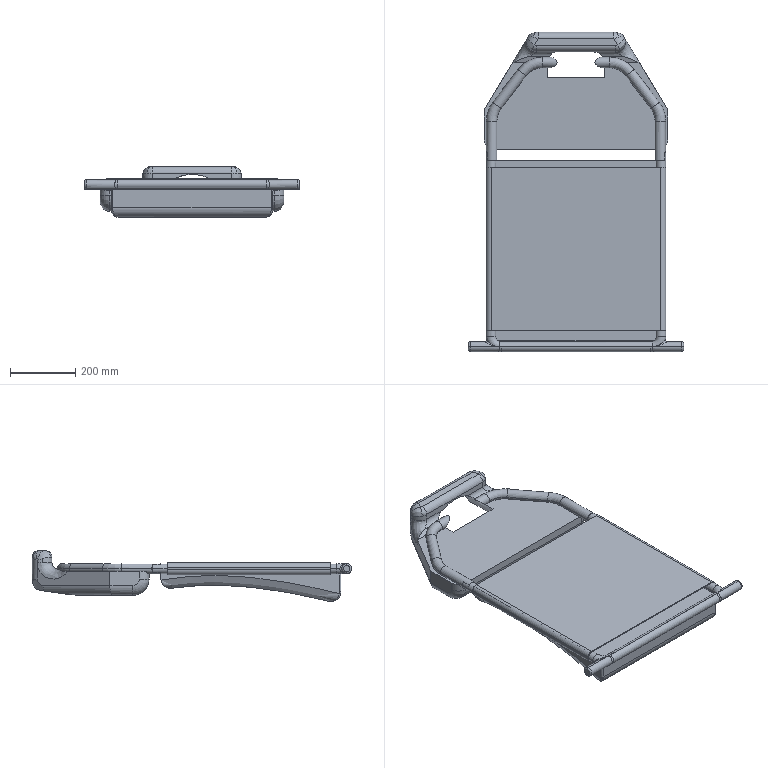Part | SolidWorks | features ICE 6, Fillet 4, Sweep 2, BossThin 1, Cut 1 | 1 solid | 165 faces | box 660 x 980.123 x 156.408 mm | volume 26120441 mm3 | cylinder 67 | plane 41 | torus 35 | spline 22 | commonest cylinder face diameters 30 x18 60 x16 32 x12 24 x8 10 x4 40 x4